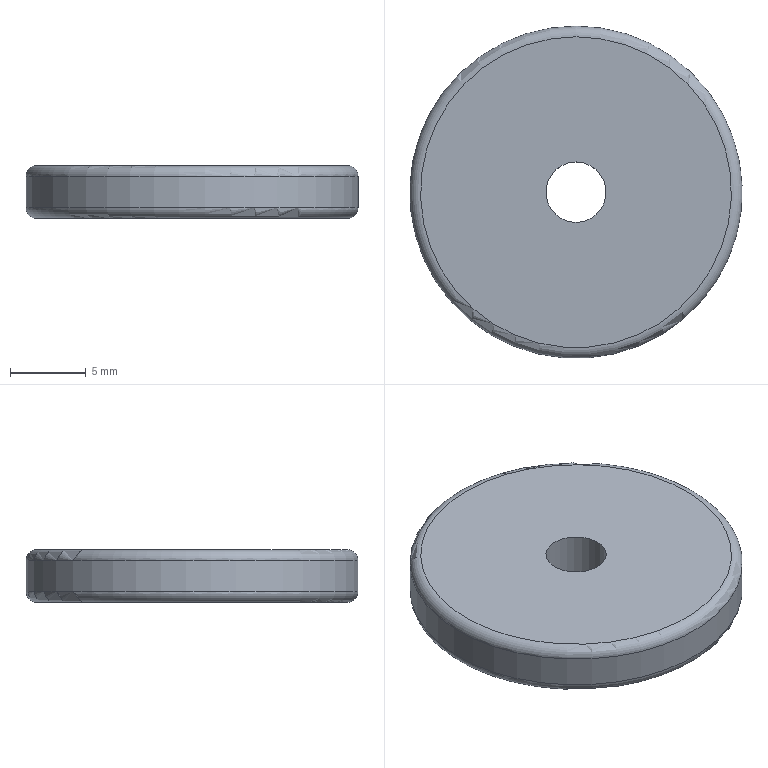Part | STEP file | 1-73.6 | 1 solid | 6 faces | box 22 x 22 x 3.5 mm | volume 1272 mm3 | cylinder 2 | plane 2 | torus 2 | commonest cylinder face diameters 4 x1 22 x1
STEP:
#1=CARTESIAN_POINT('',(0.,0.,0.));
#2=DIRECTION('',(0.,0.,1.));
#3=DIRECTION('',(1.,0.,0.));
#4=AXIS2_PLACEMENT_3D('',#1,#2,#3);
#5=CARTESIAN_POINT('',(0.,2.,0.));
#6=VERTEX_POINT('',#5);
#7=CARTESIAN_POINT('',(0.,0.,0.));
#8=DIRECTION('',(0.,0.,-1.));
#9=DIRECTION('',(0.,1.,0.));
#10=AXIS2_PLACEMENT_3D('',#7,#8,#9);
#11=CIRCLE('',#10,2.);
#12=CARTESIAN_POINT('',(0.,0.,0.));
#13=DIRECTION('',(0.,0.,-1.));
#14=DIRECTION('',(0.,1.,0.));
#15=AXIS2_PLACEMENT_3D('',#12,#13,#14);
#16=CYLINDRICAL_SURFACE('',#15,2.);
#17=CARTESIAN_POINT('',(0.,0.));
#18=DIRECTION('',(1.,0.));
#19=VECTOR('',#18,1.);
#20=LINE('',#17,#19);
#21=(GEOMETRIC_REPRESENTATION_CONTEXT(2)PARAMETRIC_REPRESENTATION_CONTEXT()REPRESENTATION_CONTEXT('',''));
#22=DEFINITIONAL_REPRESENTATION('',(#20),#21);
#23=PCURVE('',#16,#22);
#24=CARTESIAN_POINT('',(0.,-2.947,0.));
#25=DIRECTION('',(0.,0.,1.));
#26=DIRECTION('',(0.,1.,0.));
#27=AXIS2_PLACEMENT_3D('',#24,#25,#26);
#28=PLANE('',#27);
#29=CARTESIAN_POINT('',(4.947,0.));
#30=CARTESIAN_POINT('',(4.947,-3.464));
#31=CARTESIAN_POINT('',(1.947,-1.732));
#32=CARTESIAN_POINT('',(-1.053,0.));
#33=CARTESIAN_POINT('',(1.947,1.732));
#34=CARTESIAN_POINT('',(4.947,3.464));
#35=CARTESIAN_POINT('',(4.947,0.));
#36=(BOUNDED_CURVE()B_SPLINE_CURVE(2,(#29,#30,#31,#32,#33,#34,#35),.UNSPECIFIED.,.T.,.F.)B_SPLINE_CURVE_WITH_KNOTS((1,2,2,2,2,1),(-2.094,0.,2.094,4.189,6.283,8.378),.UNSPECIFIED.)CURVE()GEOMETRIC_REPRESENTATION_ITEM()RATIONAL_B_SPLINE_CURVE((1.,0.5,1.,0.5,1.,0.5,1.))REPRESENTATION_ITEM(''));
#37=(GEOMETRIC_REPRESENTATION_CONTEXT(2)PARAMETRIC_REPRESENTATION_CONTEXT()REPRESENTATION_CONTEXT('',''));
#38=DEFINITIONAL_REPRESENTATION('',(#36),#37);
#39=PCURVE('',#28,#38);
#40=SURFACE_CURVE('',#11,(#23,#39),.PCURVE_S1.);
#41=EDGE_CURVE('',#6,#6,#40,.T.);
#42=ORIENTED_EDGE('',*,*,#41,.T.);
#43=CARTESIAN_POINT('',(0.,2.,-3.5));
#44=VERTEX_POINT('',#43);
#45=CARTESIAN_POINT('',(0.,2.,0.));
#46=DIRECTION('',(0.,0.,-1.));
#47=VECTOR('',#46,1.);
#48=LINE('',#45,#47);
#49=CARTESIAN_POINT('',(6.283,0.));
#50=DIRECTION('',(0.,1.));
#51=VECTOR('',#50,1.);
#52=LINE('',#49,#51);
#53=(GEOMETRIC_REPRESENTATION_CONTEXT(2)PARAMETRIC_REPRESENTATION_CONTEXT()REPRESENTATION_CONTEXT('',''));
#54=DEFINITIONAL_REPRESENTATION('',(#52),#53);
#55=PCURVE('',#16,#54);
#56=CARTESIAN_POINT('',(0.,0.));
#57=DIRECTION('',(0.,1.));
#58=VECTOR('',#57,1.);
#59=LINE('',#56,#58);
#60=(GEOMETRIC_REPRESENTATION_CONTEXT(2)PARAMETRIC_REPRESENTATION_CONTEXT()REPRESENTATION_CONTEXT('',''));
#61=DEFINITIONAL_REPRESENTATION('',(#59),#60);
#62=PCURVE('',#16,#61);
#63=SEAM_CURVE('',#48,(#55,#62),.PCURVE_S1.);
#64=EDGE_CURVE('',#6,#44,#63,.T.);
#65=ORIENTED_EDGE('',*,*,#64,.T.);
#66=CARTESIAN_POINT('',(0.,0.,-3.5));
#67=DIRECTION('',(0.,0.,-1.));
#68=DIRECTION('',(0.,1.,0.));
#69=AXIS2_PLACEMENT_3D('',#66,#67,#68);
#70=CIRCLE('',#69,2.);
#71=CARTESIAN_POINT('',(0.,3.5));
#72=DIRECTION('',(1.,0.));
#73=VECTOR('',#72,1.);
#74=LINE('',#71,#73);
#75=(GEOMETRIC_REPRESENTATION_CONTEXT(2)PARAMETRIC_REPRESENTATION_CONTEXT()REPRESENTATION_CONTEXT('',''));
#76=DEFINITIONAL_REPRESENTATION('',(#74),#75);
#77=PCURVE('',#16,#76);
#78=CARTESIAN_POINT('',(0.,-2.947,-3.5));
#79=DIRECTION('',(0.,0.,1.));
#80=DIRECTION('',(0.,1.,0.));
#81=AXIS2_PLACEMENT_3D('',#78,#79,#80);
#82=PLANE('',#81);
#83=CARTESIAN_POINT('',(4.947,0.));
#84=CARTESIAN_POINT('',(4.947,-3.464));
#85=CARTESIAN_POINT('',(1.947,-1.732));
#86=CARTESIAN_POINT('',(-1.053,0.));
#87=CARTESIAN_POINT('',(1.947,1.732));
#88=CARTESIAN_POINT('',(4.947,3.464));
#89=CARTESIAN_POINT('',(4.947,0.));
#90=(BOUNDED_CURVE()B_SPLINE_CURVE(2,(#83,#84,#85,#86,#87,#88,#89),.UNSPECIFIED.,.T.,.F.)B_SPLINE_CURVE_WITH_KNOTS((1,2,2,2,2,1),(-2.094,0.,2.094,4.189,6.283,8.378),.UNSPECIFIED.)CURVE()GEOMETRIC_REPRESENTATION_ITEM()RATIONAL_B_SPLINE_CURVE((1.,0.5,1.,0.5,1.,0.5,1.))REPRESENTATION_ITEM(''));
#91=(GEOMETRIC_REPRESENTATION_CONTEXT(2)PARAMETRIC_REPRESENTATION_CONTEXT()REPRESENTATION_CONTEXT('',''));
#92=DEFINITIONAL_REPRESENTATION('',(#90),#91);
#93=PCURVE('',#82,#92);
#94=SURFACE_CURVE('',#70,(#77,#93),.PCURVE_S1.);
#95=EDGE_CURVE('',#44,#44,#94,.T.);
#96=ORIENTED_EDGE('',*,*,#95,.F.);
#97=ORIENTED_EDGE('',*,*,#64,.F.);
#98=EDGE_LOOP('',(#42,#65,#96,#97));
#99=FACE_BOUND('',#98,.F.);
#100=ADVANCED_FACE('',(#99),#16,.F.);
#101=CARTESIAN_POINT('',(0.,10.293,0.));
#102=VERTEX_POINT('',#101);
#103=CARTESIAN_POINT('',(0.,0.,0.));
#104=DIRECTION('',(0.,0.,1.));
#105=DIRECTION('',(0.,1.,0.));
#106=AXIS2_PLACEMENT_3D('',#103,#104,#105);
#107=CIRCLE('',#106,10.293);
#108=CARTESIAN_POINT('',(2.947,0.));
#109=DIRECTION('',(1.,0.));
#110=AXIS2_PLACEMENT_2D('',#108,#109);
#111=CIRCLE('',#110,10.293);
#112=(GEOMETRIC_REPRESENTATION_CONTEXT(2)PARAMETRIC_REPRESENTATION_CONTEXT()REPRESENTATION_CONTEXT('',''));
#113=DEFINITIONAL_REPRESENTATION('',(#111),#112);
#114=PCURVE('',#28,#113);
#115=CARTESIAN_POINT('',(0.,0.,-0.7071));
#116=DIRECTION('',(0.,0.,-1.));
#117=DIRECTION('',(0.,1.,0.));
#118=AXIS2_PLACEMENT_3D('',#115,#116,#117);
#119=TOROIDAL_SURFACE('',#118,10.293,0.7071);
#120=CARTESIAN_POINT('',(6.283,4.712));
#121=DIRECTION('',(-1.,0.));
#122=VECTOR('',#121,1.);
#123=LINE('',#120,#122);
#124=(GEOMETRIC_REPRESENTATION_CONTEXT(2)PARAMETRIC_REPRESENTATION_CONTEXT()REPRESENTATION_CONTEXT('',''));
#125=DEFINITIONAL_REPRESENTATION('',(#123),#124);
#126=PCURVE('',#119,#125);
#127=SURFACE_CURVE('',#107,(#114,#126),.PCURVE_S1.);
#128=EDGE_CURVE('',#102,#102,#127,.T.);
#129=ORIENTED_EDGE('',*,*,#128,.T.);
#130=EDGE_LOOP('',(#129));
#131=FACE_BOUND('',#130,.T.);
#132=ORIENTED_EDGE('',*,*,#41,.T.);
#133=EDGE_LOOP('',(#132));
#134=FACE_BOUND('',#133,.T.);
#135=ADVANCED_FACE('',(#131,#134),#28,.T.);
#136=CARTESIAN_POINT('',(0.,10.293,-3.5));
#137=VERTEX_POINT('',#136);
#138=CARTESIAN_POINT('',(0.,0.,-3.5));
#139=DIRECTION('',(0.,0.,1.));
#140=DIRECTION('',(0.,1.,0.));
#141=AXIS2_PLACEMENT_3D('',#138,#139,#140);
#142=CIRCLE('',#141,10.293);
#143=CARTESIAN_POINT('',(2.947,0.));
#144=DIRECTION('',(1.,0.));
#145=AXIS2_PLACEMENT_2D('',#143,#144);
#146=CIRCLE('',#145,10.293);
#147=(GEOMETRIC_REPRESENTATION_CONTEXT(2)PARAMETRIC_REPRESENTATION_CONTEXT()REPRESENTATION_CONTEXT('',''));
#148=DEFINITIONAL_REPRESENTATION('',(#146),#147);
#149=PCURVE('',#82,#148);
#150=CARTESIAN_POINT('',(0.,0.,-2.793));
#151=DIRECTION('',(0.,0.,-1.));
#152=DIRECTION('',(0.,1.,0.));
#153=AXIS2_PLACEMENT_3D('',#150,#151,#152);
#154=TOROIDAL_SURFACE('',#153,10.293,0.7071);
#155=CARTESIAN_POINT('',(6.283,1.571));
#156=DIRECTION('',(-1.,0.));
#157=VECTOR('',#156,1.);
#158=LINE('',#155,#157);
#159=(GEOMETRIC_REPRESENTATION_CONTEXT(2)PARAMETRIC_REPRESENTATION_CONTEXT()REPRESENTATION_CONTEXT('',''));
#160=DEFINITIONAL_REPRESENTATION('',(#158),#159);
#161=PCURVE('',#154,#160);
#162=SURFACE_CURVE('',#142,(#149,#161),.PCURVE_S1.);
#163=EDGE_CURVE('',#137,#137,#162,.T.);
#164=ORIENTED_EDGE('',*,*,#163,.T.);
#165=EDGE_LOOP('',(#164));
#166=FACE_BOUND('',#165,.F.);
#167=ORIENTED_EDGE('',*,*,#95,.T.);
#168=EDGE_LOOP('',(#167));
#169=FACE_BOUND('',#168,.F.);
#170=ADVANCED_FACE('',(#166,#169),#82,.F.);
#171=CARTESIAN_POINT('',(0.,11.,-0.7071));
#172=VERTEX_POINT('',#171);
#173=CARTESIAN_POINT('',(0.,0.,-0.7071));
#174=DIRECTION('',(0.,0.,1.));
#175=DIRECTION('',(0.,1.,0.));
#176=AXIS2_PLACEMENT_3D('',#173,#174,#175);
#177=CIRCLE('',#176,11.);
#178=CARTESIAN_POINT('',(0.,0.,0.));
#179=DIRECTION('',(0.,0.,-1.));
#180=DIRECTION('',(0.,1.,0.));
#181=AXIS2_PLACEMENT_3D('',#178,#179,#180);
#182=CYLINDRICAL_SURFACE('',#181,11.);
#183=CARTESIAN_POINT('',(6.283,0.7071));
#184=DIRECTION('',(-1.,0.));
#185=VECTOR('',#184,1.);
#186=LINE('',#183,#185);
#187=(GEOMETRIC_REPRESENTATION_CONTEXT(2)PARAMETRIC_REPRESENTATION_CONTEXT()REPRESENTATION_CONTEXT('',''));
#188=DEFINITIONAL_REPRESENTATION('',(#186),#187);
#189=PCURVE('',#182,#188);
#190=CARTESIAN_POINT('',(6.283,6.283));
#191=DIRECTION('',(-1.,0.));
#192=VECTOR('',#191,1.);
#193=LINE('',#190,#192);
#194=(GEOMETRIC_REPRESENTATION_CONTEXT(2)PARAMETRIC_REPRESENTATION_CONTEXT()REPRESENTATION_CONTEXT('',''));
#195=DEFINITIONAL_REPRESENTATION('',(#193),#194);
#196=PCURVE('',#119,#195);
#197=SURFACE_CURVE('',#177,(#189,#196),.PCURVE_S1.);
#198=EDGE_CURVE('',#172,#172,#197,.T.);
#199=ORIENTED_EDGE('',*,*,#198,.F.);
#200=CARTESIAN_POINT('',(0.,11.,-2.793));
#201=VERTEX_POINT('',#200);
#202=CARTESIAN_POINT('',(0.,11.,-0.7071));
#203=DIRECTION('',(0.,0.,-1.));
#204=VECTOR('',#203,1.);
#205=LINE('',#202,#204);
#206=CARTESIAN_POINT('',(6.283,0.7071));
#207=DIRECTION('',(0.,1.));
#208=VECTOR('',#207,1.);
#209=LINE('',#206,#208);
#210=(GEOMETRIC_REPRESENTATION_CONTEXT(2)PARAMETRIC_REPRESENTATION_CONTEXT()REPRESENTATION_CONTEXT('',''));
#211=DEFINITIONAL_REPRESENTATION('',(#209),#210);
#212=PCURVE('',#182,#211);
#213=CARTESIAN_POINT('',(0.,0.7071));
#214=DIRECTION('',(0.,1.));
#215=VECTOR('',#214,1.);
#216=LINE('',#213,#215);
#217=(GEOMETRIC_REPRESENTATION_CONTEXT(2)PARAMETRIC_REPRESENTATION_CONTEXT()REPRESENTATION_CONTEXT('',''));
#218=DEFINITIONAL_REPRESENTATION('',(#216),#217);
#219=PCURVE('',#182,#218);
#220=SEAM_CURVE('',#205,(#212,#219),.PCURVE_S1.);
#221=EDGE_CURVE('',#172,#201,#220,.T.);
#222=ORIENTED_EDGE('',*,*,#221,.T.);
#223=CARTESIAN_POINT('',(0.,0.,-2.793));
#224=DIRECTION('',(0.,0.,1.));
#225=DIRECTION('',(0.,1.,0.));
#226=AXIS2_PLACEMENT_3D('',#223,#224,#225);
#227=CIRCLE('',#226,11.);
#228=CARTESIAN_POINT('',(6.283,2.793));
#229=DIRECTION('',(-1.,0.));
#230=VECTOR('',#229,1.);
#231=LINE('',#228,#230);
#232=(GEOMETRIC_REPRESENTATION_CONTEXT(2)PARAMETRIC_REPRESENTATION_CONTEXT()REPRESENTATION_CONTEXT('',''));
#233=DEFINITIONAL_REPRESENTATION('',(#231),#232);
#234=PCURVE('',#182,#233);
#235=CARTESIAN_POINT('',(6.283,0.));
#236=DIRECTION('',(-1.,0.));
#237=VECTOR('',#236,1.);
#238=LINE('',#235,#237);
#239=(GEOMETRIC_REPRESENTATION_CONTEXT(2)PARAMETRIC_REPRESENTATION_CONTEXT()REPRESENTATION_CONTEXT('',''));
#240=DEFINITIONAL_REPRESENTATION('',(#238),#239);
#241=PCURVE('',#154,#240);
#242=SURFACE_CURVE('',#227,(#234,#241),.PCURVE_S1.);
#243=EDGE_CURVE('',#201,#201,#242,.T.);
#244=ORIENTED_EDGE('',*,*,#243,.T.);
#245=ORIENTED_EDGE('',*,*,#221,.F.);
#246=EDGE_LOOP('',(#199,#222,#244,#245));
#247=FACE_BOUND('',#246,.T.);
#248=ADVANCED_FACE('',(#247),#182,.T.);
#249=ORIENTED_EDGE('',*,*,#128,.F.);
#250=CARTESIAN_POINT('',(0.,10.293,-0.7071));
#251=DIRECTION('',(-1.,0.,0.));
#252=DIRECTION('',(0.,0.,1.));
#253=AXIS2_PLACEMENT_3D('',#250,#251,#252);
#254=CIRCLE('',#253,0.7071);
#255=CARTESIAN_POINT('',(6.283,4.712));
#256=DIRECTION('',(0.,1.));
#257=VECTOR('',#256,1.);
#258=LINE('',#255,#257);
#259=(GEOMETRIC_REPRESENTATION_CONTEXT(2)PARAMETRIC_REPRESENTATION_CONTEXT()REPRESENTATION_CONTEXT('',''));
#260=DEFINITIONAL_REPRESENTATION('',(#258),#259);
#261=PCURVE('',#119,#260);
#262=CARTESIAN_POINT('',(0.,4.712));
#263=DIRECTION('',(0.,1.));
#264=VECTOR('',#263,1.);
#265=LINE('',#262,#264);
#266=(GEOMETRIC_REPRESENTATION_CONTEXT(2)PARAMETRIC_REPRESENTATION_CONTEXT()REPRESENTATION_CONTEXT('',''));
#267=DEFINITIONAL_REPRESENTATION('',(#265),#266);
#268=PCURVE('',#119,#267);
#269=SEAM_CURVE('',#254,(#261,#268),.PCURVE_S1.);
#270=EDGE_CURVE('',#102,#172,#269,.T.);
#271=ORIENTED_EDGE('',*,*,#270,.T.);
#272=ORIENTED_EDGE('',*,*,#198,.T.);
#273=ORIENTED_EDGE('',*,*,#270,.F.);
#274=EDGE_LOOP('',(#249,#271,#272,#273));
#275=FACE_BOUND('',#274,.T.);
#276=ADVANCED_FACE('',(#275),#119,.T.);
#277=CARTESIAN_POINT('',(0.,10.293,-2.793));
#278=DIRECTION('',(1.,0.,0.));
#279=DIRECTION('',(0.,0.,-1.));
#280=AXIS2_PLACEMENT_3D('',#277,#278,#279);
#281=CIRCLE('',#280,0.7071);
#282=CARTESIAN_POINT('',(0.,1.571));
#283=DIRECTION('',(0.,-1.));
#284=VECTOR('',#283,1.);
#285=LINE('',#282,#284);
#286=(GEOMETRIC_REPRESENTATION_CONTEXT(2)PARAMETRIC_REPRESENTATION_CONTEXT()REPRESENTATION_CONTEXT('',''));
#287=DEFINITIONAL_REPRESENTATION('',(#285),#286);
#288=PCURVE('',#154,#287);
#289=CARTESIAN_POINT('',(6.283,1.571));
#290=DIRECTION('',(0.,-1.));
#291=VECTOR('',#290,1.);
#292=LINE('',#289,#291);
#293=(GEOMETRIC_REPRESENTATION_CONTEXT(2)PARAMETRIC_REPRESENTATION_CONTEXT()REPRESENTATION_CONTEXT('',''));
#294=DEFINITIONAL_REPRESENTATION('',(#292),#293);
#295=PCURVE('',#154,#294);
#296=SEAM_CURVE('',#281,(#288,#295),.PCURVE_S1.);
#297=EDGE_CURVE('',#137,#201,#296,.T.);
#298=ORIENTED_EDGE('',*,*,#297,.T.);
#299=ORIENTED_EDGE('',*,*,#243,.F.);
#300=ORIENTED_EDGE('',*,*,#297,.F.);
#301=ORIENTED_EDGE('',*,*,#163,.T.);
#302=EDGE_LOOP('',(#298,#299,#300,#301));
#303=FACE_BOUND('',#302,.T.);
#304=ADVANCED_FACE('',(#303),#154,.T.);
#305=CLOSED_SHELL('',(#100,#135,#170,#248,#276,#304));
#306=MANIFOLD_SOLID_BREP('',#305);
#307=(LENGTH_UNIT()NAMED_UNIT(*)SI_UNIT(.MILLI.,.METRE.));
#308=UNCERTAINTY_MEASURE_WITH_UNIT(LENGTH_MEASURE(0.0000001),#307,'','');
#309=(NAMED_UNIT(*)PLANE_ANGLE_UNIT()SI_UNIT($,.RADIAN.));
#310=(NAMED_UNIT(*)SI_UNIT($,.STERADIAN.)SOLID_ANGLE_UNIT());
#311=(GEOMETRIC_REPRESENTATION_CONTEXT(3)GLOBAL_UNCERTAINTY_ASSIGNED_CONTEXT((#308))GLOBAL_UNIT_ASSIGNED_CONTEXT((#307,#309,#310))REPRESENTATION_CONTEXT('',''));
#312=ADVANCED_BREP_SHAPE_REPRESENTATION('',(#4,#306),#311);